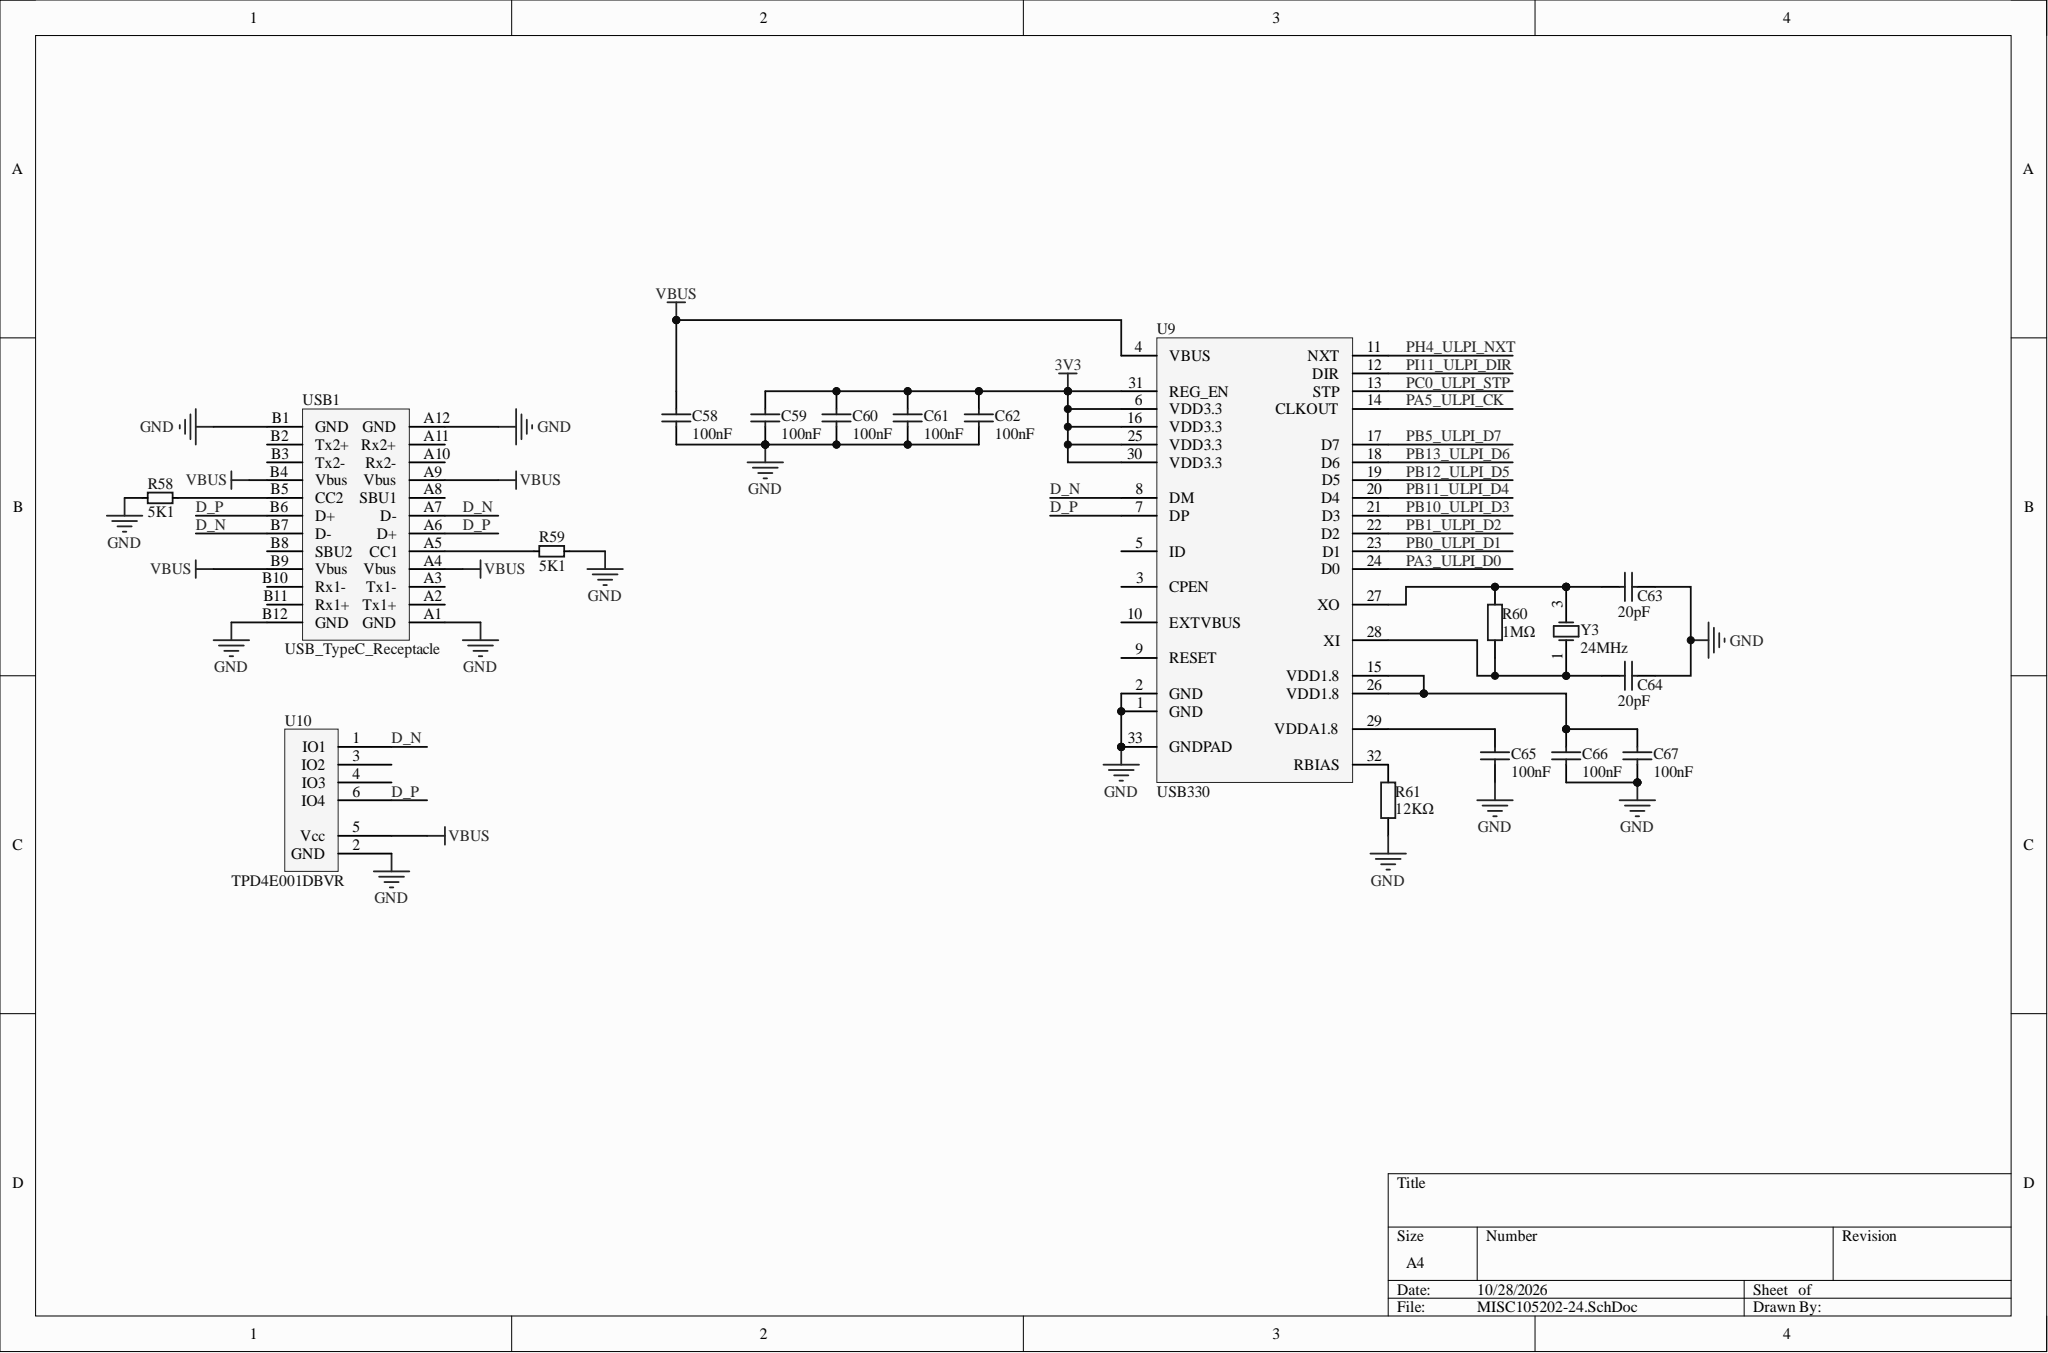Circuit board | Altium Designer | 181 parts | 141 nets | one sheet of the schematic
Parts on this sheet (reference | value | footprint):
C58 | 100nF | 0603_C
C59 | 100nF | 0603_C
C60 | 100nF | 0603_C
C61 | 100nF | 0603_C
C62 | 100nF | 0603_C
C63 | 20pF | 0402_C
C64 | 20pF | 0402_C
C65 | 100nF | 0603_C
C66 | 100nF | 0603_C
C67 | 100nF | 0603_C
R58 | 5K1 | 0402_R
R59 | 5K1 | 0402_R
R60 | 1MΩ | 0402_R
R61 | 12KΩ | 0603_R
U9 | USB330 | QFN-32_5x5x05P
U10 | TPD4E001DBVR | SOT-23-6
USB1 | USB_TypeC_Receptacle | USB_TYPEC
Y3 | 24MHz | SMD-3225_4P
Nets of these parts (net: part-pin ...):
VBUS: C58-2 U10-5 USB1-A4 USB1-A9 USB1-B4 USB1-B9 U9-4
PI11_ULPI_DIR: U9-12
PH4_ULPI_NXT: U9-11
PC0_ULPI_STP: U9-13
PB13_ULPI_D6: U9-18
PB12_ULPI_D5: U9-19
PB11_ULPI_D4: U9-20
PB10_ULPI_D3: U9-21
PB5_ULPI_D7: U9-17
PB1_ULPI_D2: U9-22
PB0_ULPI_D1: U9-23
PA5_ULPI_CK: U9-14
PA3_ULPI_D0: U9-24
NetR61_2: R61-2 U9-32
NetR59_2: R59-2 USB1-A5
NetR58_1: R58-1 USB1-B5
NetC66_2: C66-2 C67-2 U9-15 U9-26
NetC65_2: C65-2 U9-29
NetC64_1: C64-1 R60-1 Y3-1 U9-28
NetC63_1: C63-1 R60-2 Y3-3 U9-27
GND: C58-1 C59-1 C60-1 C61-1 C62-1 C63-2 C64-2 C65-1 C66-1 C67-1 R58-2 R59-1 R61-1 U10-2 USB1-A1 USB1-A12 USB1-B1 USB1-B12 U9-1 U9-2 U9-33
D_P: U10-6 USB1-A6 USB1-B6 U9-7
D_N: U10-1 USB1-A7 USB1-B7 U9-8
3V3: C59-2 C60-2 C61-2 C62-2 U9-6 U9-16 U9-25 U9-30 U9-31